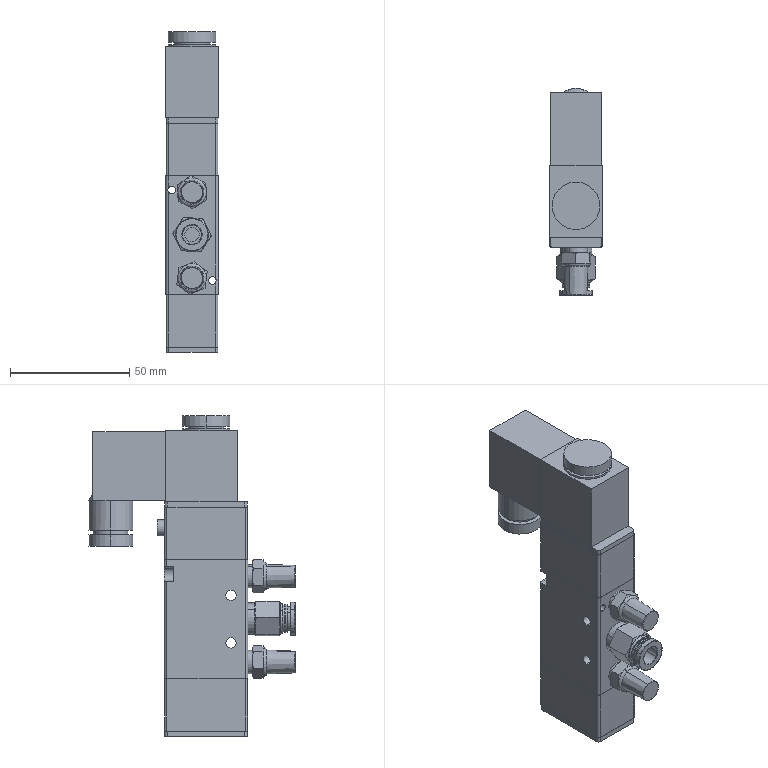Part | NX | features BREP 2 | 2 solids | 259 faces | box 22 x 86.8 x 134.6 mm | volume 119649 mm3 | plane 90 | cylinder 80 | cone 63 | torus 26 | commonest cylinder face diameters 2 x22 11.445 x6 3.2 x4 4.3 x4 4.864 x4 6 x4